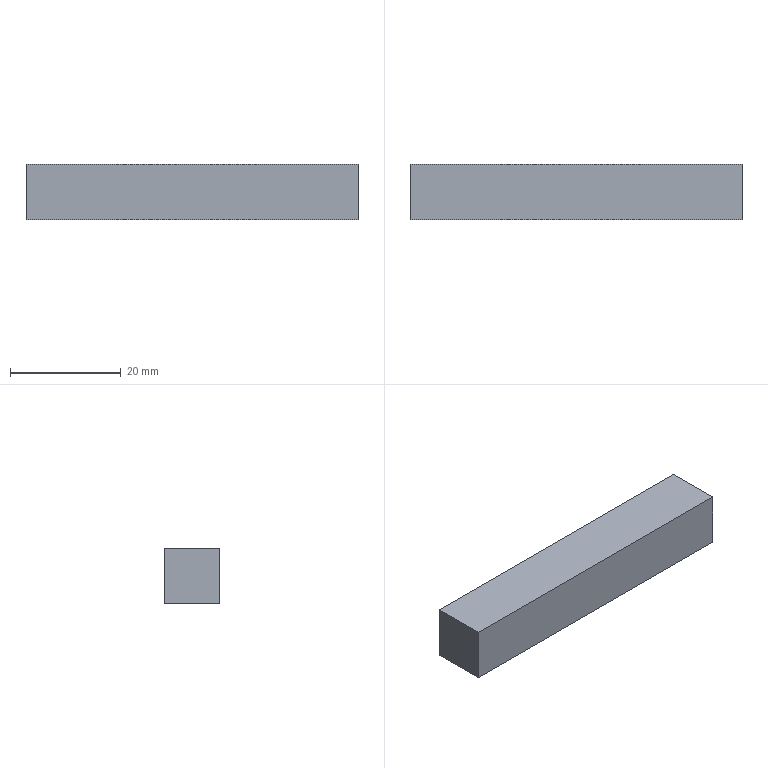Part | SolidWorks | features Extrusion 1 | 1 solid | 6 faces | box 60 x 10 x 10 mm | volume 6000 mm3 | plane 6
STEP:
#1=CARTESIAN_POINT('',(0.,5.,5.));
#2=VERTEX_POINT('',#1);
#3=CARTESIAN_POINT('',(0.,-5.,5.));
#4=VERTEX_POINT('',#3);
#5=CARTESIAN_POINT('',(0.,-5.,5.));
#6=DIRECTION('',(0.,-1.,0.));
#7=VECTOR('',#6,1000.);
#8=LINE('',#5,#7);
#9=EDGE_CURVE('',#2,#4,#8,.T.);
#10=ORIENTED_EDGE('',*,*,#9,.T.);
#11=CARTESIAN_POINT('',(60.,-5.,5.));
#12=VERTEX_POINT('',#11);
#13=CARTESIAN_POINT('',(60.,-5.,5.));
#14=DIRECTION('',(-1.,0.,0.));
#15=VECTOR('',#14,1000.);
#16=LINE('',#13,#15);
#17=EDGE_CURVE('',#12,#4,#16,.T.);
#18=ORIENTED_EDGE('',*,*,#17,.F.);
#19=CARTESIAN_POINT('',(60.,5.,5.));
#20=VERTEX_POINT('',#19);
#21=CARTESIAN_POINT('',(60.,-5.,5.));
#22=DIRECTION('',(0.,-1.,0.));
#23=VECTOR('',#22,1000.);
#24=LINE('',#21,#23);
#25=EDGE_CURVE('',#20,#12,#24,.T.);
#26=ORIENTED_EDGE('',*,*,#25,.F.);
#27=CARTESIAN_POINT('',(60.,5.,5.));
#28=DIRECTION('',(-1.,0.,0.));
#29=VECTOR('',#28,1000.);
#30=LINE('',#27,#29);
#31=EDGE_CURVE('',#20,#2,#30,.T.);
#32=ORIENTED_EDGE('',*,*,#31,.T.);
#33=EDGE_LOOP('',(#10,#18,#26,#32));
#34=FACE_OUTER_BOUND('',#33,.T.);
#35=CARTESIAN_POINT('',(60.,-5.,5.));
#36=DIRECTION('',(0.,0.,-1.));
#37=DIRECTION('',(-1.,0.,0.));
#38=AXIS2_PLACEMENT_3D('',#35,#36,#37);
#39=PLANE('',#38);
#40=ADVANCED_FACE('',(#34),#39,.F.);
#41=CARTESIAN_POINT('',(0.,-5.,-5.));
#42=VERTEX_POINT('',#41);
#43=CARTESIAN_POINT('',(0.,-5.,-5.));
#44=DIRECTION('',(0.,0.,-1.));
#45=VECTOR('',#44,1000.);
#46=LINE('',#43,#45);
#47=EDGE_CURVE('',#4,#42,#46,.T.);
#48=ORIENTED_EDGE('',*,*,#47,.T.);
#49=CARTESIAN_POINT('',(60.,-5.,-5.));
#50=VERTEX_POINT('',#49);
#51=CARTESIAN_POINT('',(60.,-5.,-5.));
#52=DIRECTION('',(-1.,0.,0.));
#53=VECTOR('',#52,1000.);
#54=LINE('',#51,#53);
#55=EDGE_CURVE('',#50,#42,#54,.T.);
#56=ORIENTED_EDGE('',*,*,#55,.F.);
#57=CARTESIAN_POINT('',(60.,-5.,-5.));
#58=DIRECTION('',(0.,0.,-1.));
#59=VECTOR('',#58,1000.);
#60=LINE('',#57,#59);
#61=EDGE_CURVE('',#12,#50,#60,.T.);
#62=ORIENTED_EDGE('',*,*,#61,.F.);
#63=ORIENTED_EDGE('',*,*,#17,.T.);
#64=EDGE_LOOP('',(#48,#56,#62,#63));
#65=FACE_OUTER_BOUND('',#64,.T.);
#66=CARTESIAN_POINT('',(60.,-5.,-5.));
#67=DIRECTION('',(0.,1.,0.));
#68=DIRECTION('',(0.,0.,1.));
#69=AXIS2_PLACEMENT_3D('',#66,#67,#68);
#70=PLANE('',#69);
#71=ADVANCED_FACE('',(#65),#70,.F.);
#72=CARTESIAN_POINT('',(0.,5.,-5.));
#73=VERTEX_POINT('',#72);
#74=CARTESIAN_POINT('',(0.,-5.,-5.));
#75=DIRECTION('',(0.,1.,0.));
#76=VECTOR('',#75,1000.);
#77=LINE('',#74,#76);
#78=EDGE_CURVE('',#42,#73,#77,.T.);
#79=ORIENTED_EDGE('',*,*,#78,.T.);
#80=CARTESIAN_POINT('',(60.,5.,-5.));
#81=VERTEX_POINT('',#80);
#82=CARTESIAN_POINT('',(60.,5.,-5.));
#83=DIRECTION('',(-1.,0.,0.));
#84=VECTOR('',#83,1000.);
#85=LINE('',#82,#84);
#86=EDGE_CURVE('',#81,#73,#85,.T.);
#87=ORIENTED_EDGE('',*,*,#86,.F.);
#88=CARTESIAN_POINT('',(60.,-5.,-5.));
#89=DIRECTION('',(0.,1.,0.));
#90=VECTOR('',#89,1000.);
#91=LINE('',#88,#90);
#92=EDGE_CURVE('',#50,#81,#91,.T.);
#93=ORIENTED_EDGE('',*,*,#92,.F.);
#94=ORIENTED_EDGE('',*,*,#55,.T.);
#95=EDGE_LOOP('',(#79,#87,#93,#94));
#96=FACE_OUTER_BOUND('',#95,.T.);
#97=CARTESIAN_POINT('',(60.,-5.,-5.));
#98=DIRECTION('',(0.,0.,1.));
#99=DIRECTION('',(1.,0.,0.));
#100=AXIS2_PLACEMENT_3D('',#97,#98,#99);
#101=PLANE('',#100);
#102=ADVANCED_FACE('',(#96),#101,.F.);
#103=CARTESIAN_POINT('',(0.,5.,-5.));
#104=DIRECTION('',(0.,0.,1.));
#105=VECTOR('',#104,1000.);
#106=LINE('',#103,#105);
#107=EDGE_CURVE('',#73,#2,#106,.T.);
#108=ORIENTED_EDGE('',*,*,#107,.T.);
#109=ORIENTED_EDGE('',*,*,#31,.F.);
#110=CARTESIAN_POINT('',(60.,5.,-5.));
#111=DIRECTION('',(0.,0.,1.));
#112=VECTOR('',#111,1000.);
#113=LINE('',#110,#112);
#114=EDGE_CURVE('',#81,#20,#113,.T.);
#115=ORIENTED_EDGE('',*,*,#114,.F.);
#116=ORIENTED_EDGE('',*,*,#86,.T.);
#117=EDGE_LOOP('',(#108,#109,#115,#116));
#118=FACE_OUTER_BOUND('',#117,.T.);
#119=CARTESIAN_POINT('',(60.,5.,-5.));
#120=DIRECTION('',(0.,-1.,0.));
#121=DIRECTION('',(0.,0.,-1.));
#122=AXIS2_PLACEMENT_3D('',#119,#120,#121);
#123=PLANE('',#122);
#124=ADVANCED_FACE('',(#118),#123,.F.);
#125=ORIENTED_EDGE('',*,*,#25,.T.);
#126=ORIENTED_EDGE('',*,*,#61,.T.);
#127=ORIENTED_EDGE('',*,*,#92,.T.);
#128=ORIENTED_EDGE('',*,*,#114,.T.);
#129=EDGE_LOOP('',(#125,#126,#127,#128));
#130=FACE_OUTER_BOUND('',#129,.T.);
#131=CARTESIAN_POINT('',(60.,0.,0.));
#132=DIRECTION('',(1.,0.,0.));
#133=DIRECTION('',(0.,0.,-1.));
#134=AXIS2_PLACEMENT_3D('',#131,#132,#133);
#135=PLANE('',#134);
#136=ADVANCED_FACE('',(#130),#135,.T.);
#137=ORIENTED_EDGE('',*,*,#9,.F.);
#138=ORIENTED_EDGE('',*,*,#107,.F.);
#139=ORIENTED_EDGE('',*,*,#78,.F.);
#140=ORIENTED_EDGE('',*,*,#47,.F.);
#141=EDGE_LOOP('',(#137,#138,#139,#140));
#142=FACE_OUTER_BOUND('',#141,.T.);
#143=CARTESIAN_POINT('',(0.,0.,0.));
#144=DIRECTION('',(1.,0.,0.));
#145=DIRECTION('',(0.,0.,-1.));
#146=AXIS2_PLACEMENT_3D('',#143,#144,#145);
#147=PLANE('',#146);
#148=ADVANCED_FACE('',(#142),#147,.F.);
#149=CLOSED_SHELL('',(#40,#71,#102,#124,#136,#148));
#150=MANIFOLD_SOLID_BREP('',#149);
#151=CARTESIAN_POINT('',(0.,0.,0.));
#152=DIRECTION('',(0.,0.,1.));
#153=DIRECTION('',(1.,0.,0.));
#154=AXIS2_PLACEMENT_3D('',#151,#152,#153);
#155=(LENGTH_UNIT()NAMED_UNIT(*)SI_UNIT(.MILLI.,.METRE.));
#156=UNCERTAINTY_MEASURE_WITH_UNIT(LENGTH_MEASURE(0.00001),#155,'','');
#157=(NAMED_UNIT(*)PLANE_ANGLE_UNIT()SI_UNIT($,.RADIAN.));
#158=(NAMED_UNIT(*)SI_UNIT($,.STERADIAN.)SOLID_ANGLE_UNIT());
#159=(GEOMETRIC_REPRESENTATION_CONTEXT(3)GLOBAL_UNCERTAINTY_ASSIGNED_CONTEXT((#156))GLOBAL_UNIT_ASSIGNED_CONTEXT((#155,#157,#158))REPRESENTATION_CONTEXT('',''));
#160=ADVANCED_BREP_SHAPE_REPRESENTATION('',(#150,#154),#159);